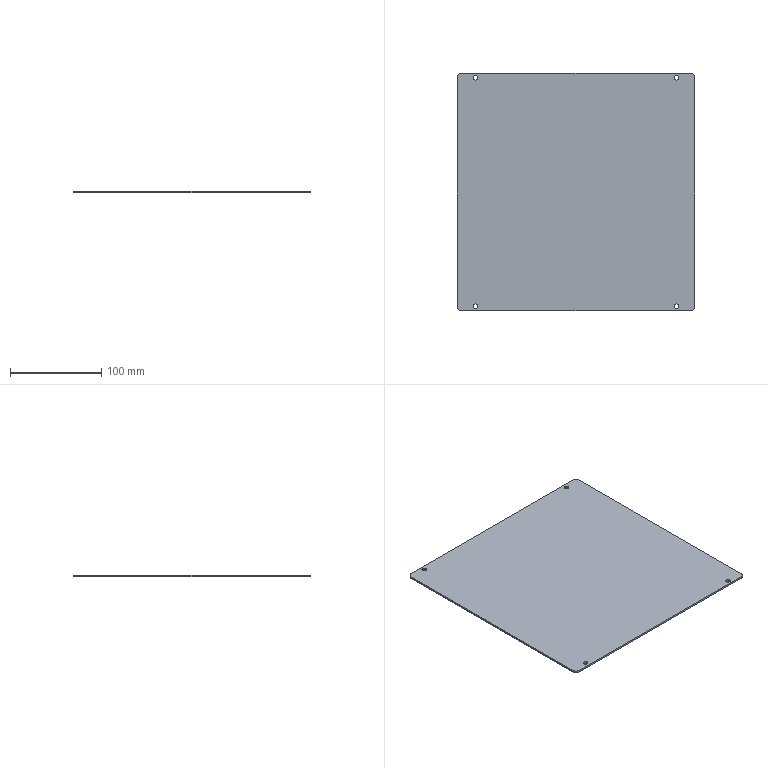Part | SolidWorks | features Extrusion 1, Fillet 1, HoleWzd 1 | 1 solid | 18 faces | box 260 x 260 x 2 mm | volume 135000 mm3 | cylinder 12 | plane 6 | commonest cylinder face diameters 5 x8 10 x4
STEP:
#1=CARTESIAN_POINT('',(-112.5,125.,0.));
#2=VERTEX_POINT('',#1);
#3=CARTESIAN_POINT('',(-107.5,125.,0.));
#4=VERTEX_POINT('',#3);
#5=CARTESIAN_POINT('',(-110.,125.,0.));
#6=DIRECTION('',(0.,0.,1.));
#7=DIRECTION('',(1.,0.,0.));
#8=AXIS2_PLACEMENT_3D('',#5,#6,#7);
#9=CIRCLE('',#8,2.5);
#10=EDGE_CURVE('',#2,#4,#9,.T.);
#11=ORIENTED_EDGE('',*,*,#10,.F.);
#12=CARTESIAN_POINT('',(-112.5,125.,2.));
#13=VERTEX_POINT('',#12);
#14=CARTESIAN_POINT('',(-112.5,125.,2.));
#15=DIRECTION('',(0.,0.,1.));
#16=VECTOR('',#15,1000.);
#17=LINE('',#14,#16);
#18=EDGE_CURVE('',#2,#13,#17,.T.);
#19=ORIENTED_EDGE('',*,*,#18,.T.);
#20=CARTESIAN_POINT('',(-107.5,125.,2.));
#21=VERTEX_POINT('',#20);
#22=CARTESIAN_POINT('',(-110.,125.,2.));
#23=DIRECTION('',(0.,0.,1.));
#24=DIRECTION('',(1.,0.,0.));
#25=AXIS2_PLACEMENT_3D('',#22,#23,#24);
#26=CIRCLE('',#25,2.5);
#27=EDGE_CURVE('',#13,#21,#26,.T.);
#28=ORIENTED_EDGE('',*,*,#27,.T.);
#29=CARTESIAN_POINT('',(-107.5,125.,2.));
#30=DIRECTION('',(0.,0.,1.));
#31=VECTOR('',#30,1000.);
#32=LINE('',#29,#31);
#33=EDGE_CURVE('',#4,#21,#32,.T.);
#34=ORIENTED_EDGE('',*,*,#33,.F.);
#35=EDGE_LOOP('',(#11,#19,#28,#34));
#36=FACE_OUTER_BOUND('',#35,.T.);
#37=CARTESIAN_POINT('',(-110.,125.,2.));
#38=DIRECTION('',(0.,0.,1.));
#39=DIRECTION('',(1.,0.,0.));
#40=AXIS2_PLACEMENT_3D('',#37,#38,#39);
#41=CYLINDRICAL_SURFACE('',#40,2.5);
#42=ADVANCED_FACE('',(#36),#41,.F.);
#43=CARTESIAN_POINT('',(-112.5,-125.,0.));
#44=VERTEX_POINT('',#43);
#45=CARTESIAN_POINT('',(-107.5,-125.,0.));
#46=VERTEX_POINT('',#45);
#47=CARTESIAN_POINT('',(-110.,-125.,0.));
#48=DIRECTION('',(0.,0.,1.));
#49=DIRECTION('',(1.,0.,0.));
#50=AXIS2_PLACEMENT_3D('',#47,#48,#49);
#51=CIRCLE('',#50,2.5);
#52=EDGE_CURVE('',#44,#46,#51,.T.);
#53=ORIENTED_EDGE('',*,*,#52,.F.);
#54=CARTESIAN_POINT('',(-112.5,-125.,2.));
#55=VERTEX_POINT('',#54);
#56=CARTESIAN_POINT('',(-112.5,-125.,2.));
#57=DIRECTION('',(0.,0.,1.));
#58=VECTOR('',#57,1000.);
#59=LINE('',#56,#58);
#60=EDGE_CURVE('',#44,#55,#59,.T.);
#61=ORIENTED_EDGE('',*,*,#60,.T.);
#62=CARTESIAN_POINT('',(-107.5,-125.,2.));
#63=VERTEX_POINT('',#62);
#64=CARTESIAN_POINT('',(-110.,-125.,2.));
#65=DIRECTION('',(0.,0.,1.));
#66=DIRECTION('',(1.,0.,0.));
#67=AXIS2_PLACEMENT_3D('',#64,#65,#66);
#68=CIRCLE('',#67,2.5);
#69=EDGE_CURVE('',#55,#63,#68,.T.);
#70=ORIENTED_EDGE('',*,*,#69,.T.);
#71=CARTESIAN_POINT('',(-107.5,-125.,2.));
#72=DIRECTION('',(0.,0.,1.));
#73=VECTOR('',#72,1000.);
#74=LINE('',#71,#73);
#75=EDGE_CURVE('',#46,#63,#74,.T.);
#76=ORIENTED_EDGE('',*,*,#75,.F.);
#77=EDGE_LOOP('',(#53,#61,#70,#76));
#78=FACE_OUTER_BOUND('',#77,.T.);
#79=CARTESIAN_POINT('',(-110.,-125.,2.));
#80=DIRECTION('',(0.,0.,1.));
#81=DIRECTION('',(1.,0.,0.));
#82=AXIS2_PLACEMENT_3D('',#79,#80,#81);
#83=CYLINDRICAL_SURFACE('',#82,2.5);
#84=ADVANCED_FACE('',(#78),#83,.F.);
#85=CARTESIAN_POINT('',(107.5,-125.,0.));
#86=VERTEX_POINT('',#85);
#87=CARTESIAN_POINT('',(112.5,-125.,0.));
#88=VERTEX_POINT('',#87);
#89=CARTESIAN_POINT('',(110.,-125.,0.));
#90=DIRECTION('',(0.,0.,1.));
#91=DIRECTION('',(1.,0.,0.));
#92=AXIS2_PLACEMENT_3D('',#89,#90,#91);
#93=CIRCLE('',#92,2.5);
#94=EDGE_CURVE('',#86,#88,#93,.T.);
#95=ORIENTED_EDGE('',*,*,#94,.F.);
#96=CARTESIAN_POINT('',(107.5,-125.,2.));
#97=VERTEX_POINT('',#96);
#98=CARTESIAN_POINT('',(107.5,-125.,2.));
#99=DIRECTION('',(0.,0.,1.));
#100=VECTOR('',#99,1000.);
#101=LINE('',#98,#100);
#102=EDGE_CURVE('',#86,#97,#101,.T.);
#103=ORIENTED_EDGE('',*,*,#102,.T.);
#104=CARTESIAN_POINT('',(112.5,-125.,2.));
#105=VERTEX_POINT('',#104);
#106=CARTESIAN_POINT('',(110.,-125.,2.));
#107=DIRECTION('',(0.,0.,1.));
#108=DIRECTION('',(1.,0.,0.));
#109=AXIS2_PLACEMENT_3D('',#106,#107,#108);
#110=CIRCLE('',#109,2.5);
#111=EDGE_CURVE('',#97,#105,#110,.T.);
#112=ORIENTED_EDGE('',*,*,#111,.T.);
#113=CARTESIAN_POINT('',(112.5,-125.,2.));
#114=DIRECTION('',(0.,0.,1.));
#115=VECTOR('',#114,1000.);
#116=LINE('',#113,#115);
#117=EDGE_CURVE('',#88,#105,#116,.T.);
#118=ORIENTED_EDGE('',*,*,#117,.F.);
#119=EDGE_LOOP('',(#95,#103,#112,#118));
#120=FACE_OUTER_BOUND('',#119,.T.);
#121=CARTESIAN_POINT('',(110.,-125.,2.));
#122=DIRECTION('',(0.,0.,1.));
#123=DIRECTION('',(1.,0.,0.));
#124=AXIS2_PLACEMENT_3D('',#121,#122,#123);
#125=CYLINDRICAL_SURFACE('',#124,2.5);
#126=ADVANCED_FACE('',(#120),#125,.F.);
#127=CARTESIAN_POINT('',(107.5,125.,0.));
#128=VERTEX_POINT('',#127);
#129=CARTESIAN_POINT('',(112.5,125.,0.));
#130=VERTEX_POINT('',#129);
#131=CARTESIAN_POINT('',(110.,125.,0.));
#132=DIRECTION('',(0.,0.,1.));
#133=DIRECTION('',(1.,0.,0.));
#134=AXIS2_PLACEMENT_3D('',#131,#132,#133);
#135=CIRCLE('',#134,2.5);
#136=EDGE_CURVE('',#128,#130,#135,.T.);
#137=ORIENTED_EDGE('',*,*,#136,.F.);
#138=CARTESIAN_POINT('',(107.5,125.,2.));
#139=VERTEX_POINT('',#138);
#140=CARTESIAN_POINT('',(107.5,125.,2.));
#141=DIRECTION('',(0.,0.,1.));
#142=VECTOR('',#141,1000.);
#143=LINE('',#140,#142);
#144=EDGE_CURVE('',#128,#139,#143,.T.);
#145=ORIENTED_EDGE('',*,*,#144,.T.);
#146=CARTESIAN_POINT('',(112.5,125.,2.));
#147=VERTEX_POINT('',#146);
#148=CARTESIAN_POINT('',(110.,125.,2.));
#149=DIRECTION('',(0.,0.,1.));
#150=DIRECTION('',(1.,0.,0.));
#151=AXIS2_PLACEMENT_3D('',#148,#149,#150);
#152=CIRCLE('',#151,2.5);
#153=EDGE_CURVE('',#139,#147,#152,.T.);
#154=ORIENTED_EDGE('',*,*,#153,.T.);
#155=CARTESIAN_POINT('',(112.5,125.,2.));
#156=DIRECTION('',(0.,0.,1.));
#157=VECTOR('',#156,1000.);
#158=LINE('',#155,#157);
#159=EDGE_CURVE('',#130,#147,#158,.T.);
#160=ORIENTED_EDGE('',*,*,#159,.F.);
#161=EDGE_LOOP('',(#137,#145,#154,#160));
#162=FACE_OUTER_BOUND('',#161,.T.);
#163=CARTESIAN_POINT('',(110.,125.,2.));
#164=DIRECTION('',(0.,0.,1.));
#165=DIRECTION('',(1.,0.,0.));
#166=AXIS2_PLACEMENT_3D('',#163,#164,#165);
#167=CYLINDRICAL_SURFACE('',#166,2.5);
#168=ADVANCED_FACE('',(#162),#167,.F.);
#169=CARTESIAN_POINT('',(130.,-125.,2.));
#170=VERTEX_POINT('',#169);
#171=CARTESIAN_POINT('',(130.,125.,2.));
#172=VERTEX_POINT('',#171);
#173=CARTESIAN_POINT('',(130.,-130.,2.));
#174=DIRECTION('',(0.,1.,0.));
#175=VECTOR('',#174,1000.);
#176=LINE('',#173,#175);
#177=EDGE_CURVE('',#170,#172,#176,.T.);
#178=ORIENTED_EDGE('',*,*,#177,.F.);
#179=CARTESIAN_POINT('',(130.,-125.,0.));
#180=VERTEX_POINT('',#179);
#181=CARTESIAN_POINT('',(130.,-125.,2.));
#182=DIRECTION('',(0.,0.,-1.));
#183=VECTOR('',#182,1000.);
#184=LINE('',#181,#183);
#185=EDGE_CURVE('',#170,#180,#184,.T.);
#186=ORIENTED_EDGE('',*,*,#185,.T.);
#187=CARTESIAN_POINT('',(130.,125.,0.));
#188=VERTEX_POINT('',#187);
#189=CARTESIAN_POINT('',(130.,-130.,0.));
#190=DIRECTION('',(0.,1.,0.));
#191=VECTOR('',#190,1000.);
#192=LINE('',#189,#191);
#193=EDGE_CURVE('',#180,#188,#192,.T.);
#194=ORIENTED_EDGE('',*,*,#193,.T.);
#195=CARTESIAN_POINT('',(130.,125.,2.));
#196=DIRECTION('',(0.,0.,1.));
#197=VECTOR('',#196,1000.);
#198=LINE('',#195,#197);
#199=EDGE_CURVE('',#188,#172,#198,.T.);
#200=ORIENTED_EDGE('',*,*,#199,.T.);
#201=EDGE_LOOP('',(#178,#186,#194,#200));
#202=FACE_OUTER_BOUND('',#201,.T.);
#203=CARTESIAN_POINT('',(130.,-130.,2.));
#204=DIRECTION('',(-1.,0.,0.));
#205=DIRECTION('',(0.,0.,1.));
#206=AXIS2_PLACEMENT_3D('',#203,#204,#205);
#207=PLANE('',#206);
#208=ADVANCED_FACE('',(#202),#207,.F.);
#209=CARTESIAN_POINT('',(125.,130.,0.));
#210=VERTEX_POINT('',#209);
#211=CARTESIAN_POINT('',(-125.,130.,0.));
#212=VERTEX_POINT('',#211);
#213=CARTESIAN_POINT('',(-130.,130.,0.));
#214=DIRECTION('',(-1.,0.,0.));
#215=VECTOR('',#214,1000.);
#216=LINE('',#213,#215);
#217=EDGE_CURVE('',#210,#212,#216,.T.);
#218=ORIENTED_EDGE('',*,*,#217,.T.);
#219=CARTESIAN_POINT('',(-125.,130.,2.));
#220=VERTEX_POINT('',#219);
#221=CARTESIAN_POINT('',(-125.,130.,2.));
#222=DIRECTION('',(0.,0.,1.));
#223=VECTOR('',#222,1000.);
#224=LINE('',#221,#223);
#225=EDGE_CURVE('',#212,#220,#224,.T.);
#226=ORIENTED_EDGE('',*,*,#225,.T.);
#227=CARTESIAN_POINT('',(125.,130.,2.));
#228=VERTEX_POINT('',#227);
#229=CARTESIAN_POINT('',(-130.,130.,2.));
#230=DIRECTION('',(-1.,0.,0.));
#231=VECTOR('',#230,1000.);
#232=LINE('',#229,#231);
#233=EDGE_CURVE('',#228,#220,#232,.T.);
#234=ORIENTED_EDGE('',*,*,#233,.F.);
#235=CARTESIAN_POINT('',(125.,130.,2.));
#236=DIRECTION('',(0.,0.,-1.));
#237=VECTOR('',#236,1000.);
#238=LINE('',#235,#237);
#239=EDGE_CURVE('',#228,#210,#238,.T.);
#240=ORIENTED_EDGE('',*,*,#239,.T.);
#241=EDGE_LOOP('',(#218,#226,#234,#240));
#242=FACE_OUTER_BOUND('',#241,.T.);
#243=CARTESIAN_POINT('',(-130.,130.,2.));
#244=DIRECTION('',(0.,-1.,0.));
#245=DIRECTION('',(0.,0.,-1.));
#246=AXIS2_PLACEMENT_3D('',#243,#244,#245);
#247=PLANE('',#246);
#248=ADVANCED_FACE('',(#242),#247,.F.);
#249=CARTESIAN_POINT('',(-130.,125.,0.));
#250=VERTEX_POINT('',#249);
#251=CARTESIAN_POINT('',(-130.,-125.,0.));
#252=VERTEX_POINT('',#251);
#253=CARTESIAN_POINT('',(-130.,-130.,0.));
#254=DIRECTION('',(0.,-1.,0.));
#255=VECTOR('',#254,1000.);
#256=LINE('',#253,#255);
#257=EDGE_CURVE('',#250,#252,#256,.T.);
#258=ORIENTED_EDGE('',*,*,#257,.T.);
#259=CARTESIAN_POINT('',(-130.,-125.,2.));
#260=VERTEX_POINT('',#259);
#261=CARTESIAN_POINT('',(-130.,-125.,2.));
#262=DIRECTION('',(0.,0.,1.));
#263=VECTOR('',#262,1000.);
#264=LINE('',#261,#263);
#265=EDGE_CURVE('',#252,#260,#264,.T.);
#266=ORIENTED_EDGE('',*,*,#265,.T.);
#267=CARTESIAN_POINT('',(-130.,125.,2.));
#268=VERTEX_POINT('',#267);
#269=CARTESIAN_POINT('',(-130.,-130.,2.));
#270=DIRECTION('',(0.,-1.,0.));
#271=VECTOR('',#270,1000.);
#272=LINE('',#269,#271);
#273=EDGE_CURVE('',#268,#260,#272,.T.);
#274=ORIENTED_EDGE('',*,*,#273,.F.);
#275=CARTESIAN_POINT('',(-130.,125.,2.));
#276=DIRECTION('',(0.,0.,-1.));
#277=VECTOR('',#276,1000.);
#278=LINE('',#275,#277);
#279=EDGE_CURVE('',#268,#250,#278,.T.);
#280=ORIENTED_EDGE('',*,*,#279,.T.);
#281=EDGE_LOOP('',(#258,#266,#274,#280));
#282=FACE_OUTER_BOUND('',#281,.T.);
#283=CARTESIAN_POINT('',(-130.,-130.,2.));
#284=DIRECTION('',(1.,0.,0.));
#285=DIRECTION('',(0.,0.,-1.));
#286=AXIS2_PLACEMENT_3D('',#283,#284,#285);
#287=PLANE('',#286);
#288=ADVANCED_FACE('',(#282),#287,.F.);
#289=CARTESIAN_POINT('',(-125.,-130.,0.));
#290=VERTEX_POINT('',#289);
#291=CARTESIAN_POINT('',(125.,-130.,0.));
#292=VERTEX_POINT('',#291);
#293=CARTESIAN_POINT('',(-130.,-130.,0.));
#294=DIRECTION('',(1.,0.,0.));
#295=VECTOR('',#294,1000.);
#296=LINE('',#293,#295);
#297=EDGE_CURVE('',#290,#292,#296,.T.);
#298=ORIENTED_EDGE('',*,*,#297,.T.);
#299=CARTESIAN_POINT('',(125.,-130.,2.));
#300=VERTEX_POINT('',#299);
#301=CARTESIAN_POINT('',(125.,-130.,2.));
#302=DIRECTION('',(0.,0.,1.));
#303=VECTOR('',#302,1000.);
#304=LINE('',#301,#303);
#305=EDGE_CURVE('',#292,#300,#304,.T.);
#306=ORIENTED_EDGE('',*,*,#305,.T.);
#307=CARTESIAN_POINT('',(-125.,-130.,2.));
#308=VERTEX_POINT('',#307);
#309=CARTESIAN_POINT('',(-130.,-130.,2.));
#310=DIRECTION('',(1.,0.,0.));
#311=VECTOR('',#310,1000.);
#312=LINE('',#309,#311);
#313=EDGE_CURVE('',#308,#300,#312,.T.);
#314=ORIENTED_EDGE('',*,*,#313,.F.);
#315=CARTESIAN_POINT('',(-125.,-130.,2.));
#316=DIRECTION('',(0.,0.,-1.));
#317=VECTOR('',#316,1000.);
#318=LINE('',#315,#317);
#319=EDGE_CURVE('',#308,#290,#318,.T.);
#320=ORIENTED_EDGE('',*,*,#319,.T.);
#321=EDGE_LOOP('',(#298,#306,#314,#320));
#322=FACE_OUTER_BOUND('',#321,.T.);
#323=CARTESIAN_POINT('',(-130.,-130.,2.));
#324=DIRECTION('',(0.,1.,0.));
#325=DIRECTION('',(0.,0.,1.));
#326=AXIS2_PLACEMENT_3D('',#323,#324,#325);
#327=PLANE('',#326);
#328=ADVANCED_FACE('',(#322),#327,.F.);
#329=CARTESIAN_POINT('',(-110.,125.,2.));
#330=DIRECTION('',(0.,0.,1.));
#331=DIRECTION('',(1.,0.,0.));
#332=AXIS2_PLACEMENT_3D('',#329,#330,#331);
#333=CIRCLE('',#332,2.5);
#334=EDGE_CURVE('',#21,#13,#333,.T.);
#335=ORIENTED_EDGE('',*,*,#334,.F.);
#336=ORIENTED_EDGE('',*,*,#27,.F.);
#337=EDGE_LOOP('',(#335,#336));
#338=FACE_BOUND('',#337,.T.);
#339=CARTESIAN_POINT('',(-110.,-125.,2.));
#340=DIRECTION('',(0.,0.,1.));
#341=DIRECTION('',(1.,0.,0.));
#342=AXIS2_PLACEMENT_3D('',#339,#340,#341);
#343=CIRCLE('',#342,2.5);
#344=EDGE_CURVE('',#63,#55,#343,.T.);
#345=ORIENTED_EDGE('',*,*,#344,.F.);
#346=ORIENTED_EDGE('',*,*,#69,.F.);
#347=EDGE_LOOP('',(#345,#346));
#348=FACE_BOUND('',#347,.T.);
#349=CARTESIAN_POINT('',(110.,-125.,2.));
#350=DIRECTION('',(0.,0.,1.));
#351=DIRECTION('',(1.,0.,0.));
#352=AXIS2_PLACEMENT_3D('',#349,#350,#351);
#353=CIRCLE('',#352,2.5);
#354=EDGE_CURVE('',#105,#97,#353,.T.);
#355=ORIENTED_EDGE('',*,*,#354,.F.);
#356=ORIENTED_EDGE('',*,*,#111,.F.);
#357=EDGE_LOOP('',(#355,#356));
#358=FACE_BOUND('',#357,.T.);
#359=CARTESIAN_POINT('',(110.,125.,2.));
#360=DIRECTION('',(0.,0.,1.));
#361=DIRECTION('',(1.,0.,0.));
#362=AXIS2_PLACEMENT_3D('',#359,#360,#361);
#363=CIRCLE('',#362,2.5);
#364=EDGE_CURVE('',#147,#139,#363,.T.);
#365=ORIENTED_EDGE('',*,*,#364,.F.);
#366=ORIENTED_EDGE('',*,*,#153,.F.);
#367=EDGE_LOOP('',(#365,#366));
#368=FACE_BOUND('',#367,.T.);
#369=ORIENTED_EDGE('',*,*,#313,.T.);
#370=CARTESIAN_POINT('',(125.,-125.,2.));
#371=DIRECTION('',(0.,0.,1.));
#372=DIRECTION('',(-1.,0.,0.));
#373=AXIS2_PLACEMENT_3D('',#370,#371,#372);
#374=CIRCLE('',#373,5.);
#375=EDGE_CURVE('',#300,#170,#374,.T.);
#376=ORIENTED_EDGE('',*,*,#375,.T.);
#377=ORIENTED_EDGE('',*,*,#177,.T.);
#378=CARTESIAN_POINT('',(125.,125.,2.));
#379=DIRECTION('',(0.,0.,1.));
#380=DIRECTION('',(-1.,0.,0.));
#381=AXIS2_PLACEMENT_3D('',#378,#379,#380);
#382=CIRCLE('',#381,5.);
#383=EDGE_CURVE('',#172,#228,#382,.T.);
#384=ORIENTED_EDGE('',*,*,#383,.T.);
#385=ORIENTED_EDGE('',*,*,#233,.T.);
#386=CARTESIAN_POINT('',(-125.,125.,2.));
#387=DIRECTION('',(0.,0.,1.));
#388=DIRECTION('',(-1.,0.,0.));
#389=AXIS2_PLACEMENT_3D('',#386,#387,#388);
#390=CIRCLE('',#389,5.);
#391=EDGE_CURVE('',#220,#268,#390,.T.);
#392=ORIENTED_EDGE('',*,*,#391,.T.);
#393=ORIENTED_EDGE('',*,*,#273,.T.);
#394=CARTESIAN_POINT('',(-125.,-125.,2.));
#395=DIRECTION('',(0.,0.,1.));
#396=DIRECTION('',(-1.,0.,0.));
#397=AXIS2_PLACEMENT_3D('',#394,#395,#396);
#398=CIRCLE('',#397,5.);
#399=EDGE_CURVE('',#260,#308,#398,.T.);
#400=ORIENTED_EDGE('',*,*,#399,.T.);
#401=EDGE_LOOP('',(#369,#376,#377,#384,#385,#392,#393,#400));
#402=FACE_OUTER_BOUND('',#401,.T.);
#403=CARTESIAN_POINT('',(0.,0.,2.));
#404=DIRECTION('',(0.,0.,-1.));
#405=DIRECTION('',(-1.,0.,0.));
#406=AXIS2_PLACEMENT_3D('',#403,#404,#405);
#407=PLANE('',#406);
#408=ADVANCED_FACE('',(#338,#348,#358,#368,#402),#407,.F.);
#409=CARTESIAN_POINT('',(-110.,125.,0.));
#410=DIRECTION('',(0.,0.,1.));
#411=DIRECTION('',(1.,0.,0.));
#412=AXIS2_PLACEMENT_3D('',#409,#410,#411);
#413=CIRCLE('',#412,2.5);
#414=EDGE_CURVE('',#4,#2,#413,.T.);
#415=ORIENTED_EDGE('',*,*,#414,.T.);
#416=ORIENTED_EDGE('',*,*,#10,.T.);
#417=EDGE_LOOP('',(#415,#416));
#418=FACE_BOUND('',#417,.T.);
#419=CARTESIAN_POINT('',(-110.,-125.,0.));
#420=DIRECTION('',(0.,0.,1.));
#421=DIRECTION('',(1.,0.,0.));
#422=AXIS2_PLACEMENT_3D('',#419,#420,#421);
#423=CIRCLE('',#422,2.5);
#424=EDGE_CURVE('',#46,#44,#423,.T.);
#425=ORIENTED_EDGE('',*,*,#424,.T.);
#426=ORIENTED_EDGE('',*,*,#52,.T.);
#427=EDGE_LOOP('',(#425,#426));
#428=FACE_BOUND('',#427,.T.);
#429=CARTESIAN_POINT('',(110.,-125.,0.));
#430=DIRECTION('',(0.,0.,1.));
#431=DIRECTION('',(1.,0.,0.));
#432=AXIS2_PLACEMENT_3D('',#429,#430,#431);
#433=CIRCLE('',#432,2.5);
#434=EDGE_CURVE('',#88,#86,#433,.T.);
#435=ORIENTED_EDGE('',*,*,#434,.T.);
#436=ORIENTED_EDGE('',*,*,#94,.T.);
#437=EDGE_LOOP('',(#435,#436));
#438=FACE_BOUND('',#437,.T.);
#439=CARTESIAN_POINT('',(110.,125.,0.));
#440=DIRECTION('',(0.,0.,1.));
#441=DIRECTION('',(1.,0.,0.));
#442=AXIS2_PLACEMENT_3D('',#439,#440,#441);
#443=CIRCLE('',#442,2.5);
#444=EDGE_CURVE('',#130,#128,#443,.T.);
#445=ORIENTED_EDGE('',*,*,#444,.T.);
#446=ORIENTED_EDGE('',*,*,#136,.T.);
#447=EDGE_LOOP('',(#445,#446));
#448=FACE_BOUND('',#447,.T.);
#449=ORIENTED_EDGE('',*,*,#193,.F.);
#450=CARTESIAN_POINT('',(125.,-125.,0.));
#451=DIRECTION('',(0.,0.,-1.));
#452=DIRECTION('',(-1.,0.,0.));
#453=AXIS2_PLACEMENT_3D('',#450,#451,#452);
#454=CIRCLE('',#453,5.);
#455=EDGE_CURVE('',#180,#292,#454,.T.);
#456=ORIENTED_EDGE('',*,*,#455,.T.);
#457=ORIENTED_EDGE('',*,*,#297,.F.);
#458=CARTESIAN_POINT('',(-125.,-125.,0.));
#459=DIRECTION('',(0.,0.,-1.));
#460=DIRECTION('',(-1.,0.,0.));
#461=AXIS2_PLACEMENT_3D('',#458,#459,#460);
#462=CIRCLE('',#461,5.);
#463=EDGE_CURVE('',#290,#252,#462,.T.);
#464=ORIENTED_EDGE('',*,*,#463,.T.);
#465=ORIENTED_EDGE('',*,*,#257,.F.);
#466=CARTESIAN_POINT('',(-125.,125.,0.));
#467=DIRECTION('',(0.,0.,-1.));
#468=DIRECTION('',(-1.,0.,0.));
#469=AXIS2_PLACEMENT_3D('',#466,#467,#468);
#470=CIRCLE('',#469,5.);
#471=EDGE_CURVE('',#250,#212,#470,.T.);
#472=ORIENTED_EDGE('',*,*,#471,.T.);
#473=ORIENTED_EDGE('',*,*,#217,.F.);
#474=CARTESIAN_POINT('',(125.,125.,0.));
#475=DIRECTION('',(0.,0.,-1.));
#476=DIRECTION('',(-1.,0.,0.));
#477=AXIS2_PLACEMENT_3D('',#474,#475,#476);
#478=CIRCLE('',#477,5.);
#479=EDGE_CURVE('',#210,#188,#478,.T.);
#480=ORIENTED_EDGE('',*,*,#479,.T.);
#481=EDGE_LOOP('',(#449,#456,#457,#464,#465,#472,#473,#480));
#482=FACE_OUTER_BOUND('',#481,.T.);
#483=CARTESIAN_POINT('',(0.,0.,0.));
#484=DIRECTION('',(0.,0.,-1.));
#485=DIRECTION('',(-1.,0.,0.));
#486=AXIS2_PLACEMENT_3D('',#483,#484,#485);
#487=PLANE('',#486);
#488=ADVANCED_FACE('',(#418,#428,#438,#448,#482),#487,.T.);
#489=ORIENTED_EDGE('',*,*,#375,.F.);
#490=ORIENTED_EDGE('',*,*,#305,.F.);
#491=ORIENTED_EDGE('',*,*,#455,.F.);
#492=ORIENTED_EDGE('',*,*,#185,.F.);
#493=EDGE_LOOP('',(#489,#490,#491,#492));
#494=FACE_OUTER_BOUND('',#493,.T.);
#495=CARTESIAN_POINT('',(125.,-125.,2.));
#496=DIRECTION('',(0.,0.,-1.));
#497=DIRECTION('',(-1.,0.,0.));
#498=AXIS2_PLACEMENT_3D('',#495,#496,#497);
#499=CYLINDRICAL_SURFACE('',#498,5.);
#500=ADVANCED_FACE('',(#494),#499,.T.);
#501=ORIENTED_EDGE('',*,*,#399,.F.);
#502=ORIENTED_EDGE('',*,*,#265,.F.);
#503=ORIENTED_EDGE('',*,*,#463,.F.);
#504=ORIENTED_EDGE('',*,*,#319,.F.);
#505=EDGE_LOOP('',(#501,#502,#503,#504));
#506=FACE_OUTER_BOUND('',#505,.T.);
#507=CARTESIAN_POINT('',(-125.,-125.,2.));
#508=DIRECTION('',(0.,0.,-1.));
#509=DIRECTION('',(-1.,0.,0.));
#510=AXIS2_PLACEMENT_3D('',#507,#508,#509);
#511=CYLINDRICAL_SURFACE('',#510,5.);
#512=ADVANCED_FACE('',(#506),#511,.T.);
#513=ORIENTED_EDGE('',*,*,#391,.F.);
#514=ORIENTED_EDGE('',*,*,#225,.F.);
#515=ORIENTED_EDGE('',*,*,#471,.F.);
#516=ORIENTED_EDGE('',*,*,#279,.F.);
#517=EDGE_LOOP('',(#513,#514,#515,#516));
#518=FACE_OUTER_BOUND('',#517,.T.);
#519=CARTESIAN_POINT('',(-125.,125.,2.));
#520=DIRECTION('',(0.,0.,-1.));
#521=DIRECTION('',(-1.,0.,0.));
#522=AXIS2_PLACEMENT_3D('',#519,#520,#521);
#523=CYLINDRICAL_SURFACE('',#522,5.);
#524=ADVANCED_FACE('',(#518),#523,.T.);
#525=ORIENTED_EDGE('',*,*,#383,.F.);
#526=ORIENTED_EDGE('',*,*,#199,.F.);
#527=ORIENTED_EDGE('',*,*,#479,.F.);
#528=ORIENTED_EDGE('',*,*,#239,.F.);
#529=EDGE_LOOP('',(#525,#526,#527,#528));
#530=FACE_OUTER_BOUND('',#529,.T.);
#531=CARTESIAN_POINT('',(125.,125.,2.));
#532=DIRECTION('',(0.,0.,-1.));
#533=DIRECTION('',(-1.,0.,0.));
#534=AXIS2_PLACEMENT_3D('',#531,#532,#533);
#535=CYLINDRICAL_SURFACE('',#534,5.);
#536=ADVANCED_FACE('',(#530),#535,.T.);
#537=ORIENTED_EDGE('',*,*,#144,.F.);
#538=ORIENTED_EDGE('',*,*,#444,.F.);
#539=ORIENTED_EDGE('',*,*,#159,.T.);
#540=ORIENTED_EDGE('',*,*,#364,.T.);
#541=EDGE_LOOP('',(#537,#538,#539,#540));
#542=FACE_OUTER_BOUND('',#541,.T.);
#543=CARTESIAN_POINT('',(110.,125.,2.));
#544=DIRECTION('',(0.,0.,1.));
#545=DIRECTION('',(1.,0.,0.));
#546=AXIS2_PLACEMENT_3D('',#543,#544,#545);
#547=CYLINDRICAL_SURFACE('',#546,2.5);
#548=ADVANCED_FACE('',(#542),#547,.F.);
#549=ORIENTED_EDGE('',*,*,#102,.F.);
#550=ORIENTED_EDGE('',*,*,#434,.F.);
#551=ORIENTED_EDGE('',*,*,#117,.T.);
#552=ORIENTED_EDGE('',*,*,#354,.T.);
#553=EDGE_LOOP('',(#549,#550,#551,#552));
#554=FACE_OUTER_BOUND('',#553,.T.);
#555=CARTESIAN_POINT('',(110.,-125.,2.));
#556=DIRECTION('',(0.,0.,1.));
#557=DIRECTION('',(1.,0.,0.));
#558=AXIS2_PLACEMENT_3D('',#555,#556,#557);
#559=CYLINDRICAL_SURFACE('',#558,2.5);
#560=ADVANCED_FACE('',(#554),#559,.F.);
#561=ORIENTED_EDGE('',*,*,#60,.F.);
#562=ORIENTED_EDGE('',*,*,#424,.F.);
#563=ORIENTED_EDGE('',*,*,#75,.T.);
#564=ORIENTED_EDGE('',*,*,#344,.T.);
#565=EDGE_LOOP('',(#561,#562,#563,#564));
#566=FACE_OUTER_BOUND('',#565,.T.);
#567=CARTESIAN_POINT('',(-110.,-125.,2.));
#568=DIRECTION('',(0.,0.,1.));
#569=DIRECTION('',(1.,0.,0.));
#570=AXIS2_PLACEMENT_3D('',#567,#568,#569);
#571=CYLINDRICAL_SURFACE('',#570,2.5);
#572=ADVANCED_FACE('',(#566),#571,.F.);
#573=ORIENTED_EDGE('',*,*,#18,.F.);
#574=ORIENTED_EDGE('',*,*,#414,.F.);
#575=ORIENTED_EDGE('',*,*,#33,.T.);
#576=ORIENTED_EDGE('',*,*,#334,.T.);
#577=EDGE_LOOP('',(#573,#574,#575,#576));
#578=FACE_OUTER_BOUND('',#577,.T.);
#579=CARTESIAN_POINT('',(-110.,125.,2.));
#580=DIRECTION('',(0.,0.,1.));
#581=DIRECTION('',(1.,0.,0.));
#582=AXIS2_PLACEMENT_3D('',#579,#580,#581);
#583=CYLINDRICAL_SURFACE('',#582,2.5);
#584=ADVANCED_FACE('',(#578),#583,.F.);
#585=CLOSED_SHELL('',(#42,#84,#126,#168,#208,#248,#288,#328,#408,#488,#500,#512,#524,#536,#548,#560,#572,#584));
#586=MANIFOLD_SOLID_BREP('',#585);
#587=CARTESIAN_POINT('',(0.,0.,0.));
#588=DIRECTION('',(0.,0.,1.));
#589=DIRECTION('',(1.,0.,0.));
#590=AXIS2_PLACEMENT_3D('',#587,#588,#589);
#591=(LENGTH_UNIT()NAMED_UNIT(*)SI_UNIT(.MILLI.,.METRE.));
#592=UNCERTAINTY_MEASURE_WITH_UNIT(LENGTH_MEASURE(0.00001),#591,'','');
#593=(NAMED_UNIT(*)PLANE_ANGLE_UNIT()SI_UNIT($,.RADIAN.));
#594=(NAMED_UNIT(*)SI_UNIT($,.STERADIAN.)SOLID_ANGLE_UNIT());
#595=(GEOMETRIC_REPRESENTATION_CONTEXT(3)GLOBAL_UNCERTAINTY_ASSIGNED_CONTEXT((#592))GLOBAL_UNIT_ASSIGNED_CONTEXT((#591,#593,#594))REPRESENTATION_CONTEXT('',''));
#596=ADVANCED_BREP_SHAPE_REPRESENTATION('',(#586,#590),#595);